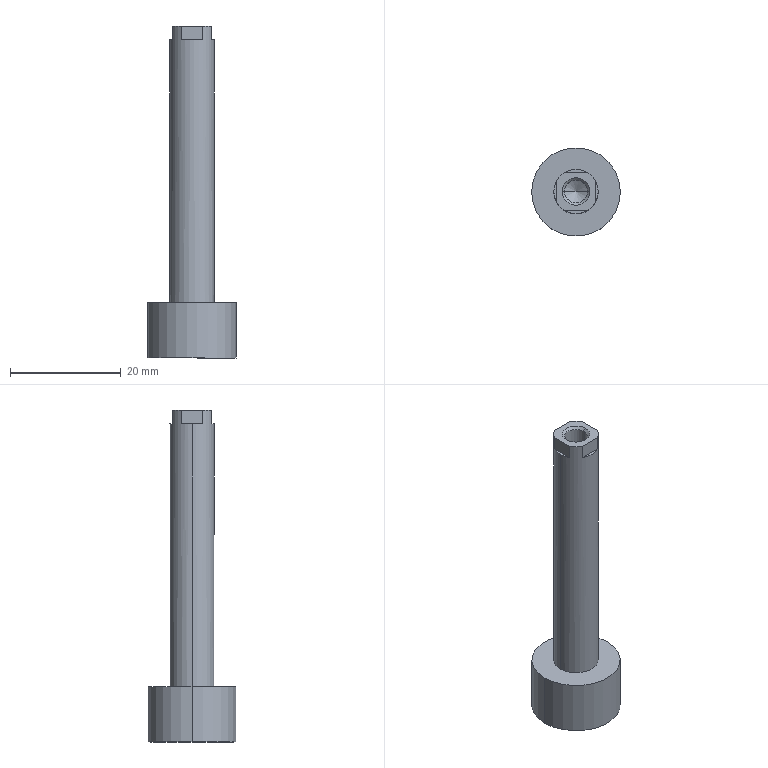Part | STEP file | 1 solid | 21 faces | box 16 x 16 x 60 mm | volume 4417 mm3 | plane 11 | cylinder 6 | cone 4 | commonest cylinder face diameters 4.134 x2 8 x2 16 x2
STEP:
#1=CARTESIAN_POINT('',(-4.,0.,-27.5));
#2=VERTEX_POINT('',#1);
#3=CARTESIAN_POINT('',(-4.,0.,20.));
#4=VERTEX_POINT('',#3);
#5=CARTESIAN_POINT('',(-4.,0.,-27.5));
#6=DIRECTION('',(0.,0.,1.));
#7=VECTOR('',#6,1000.);
#8=LINE('',#5,#7);
#9=EDGE_CURVE('',#2,#4,#8,.T.);
#10=ORIENTED_EDGE('',*,*,#9,.F.);
#11=CARTESIAN_POINT('',(4.,0.,-27.5));
#12=VERTEX_POINT('',#11);
#13=CARTESIAN_POINT('',(0.,0.,-27.5));
#14=DIRECTION('',(0.,0.,1.));
#15=DIRECTION('',(1.,0.,0.));
#16=AXIS2_PLACEMENT_3D('',#13,#14,#15);
#17=CIRCLE('',#16,4.);
#18=EDGE_CURVE('',#2,#12,#17,.T.);
#19=ORIENTED_EDGE('',*,*,#18,.T.);
#20=CARTESIAN_POINT('',(4.,0.,20.));
#21=VERTEX_POINT('',#20);
#22=CARTESIAN_POINT('',(4.,0.,-27.5));
#23=DIRECTION('',(0.,0.,1.));
#24=VECTOR('',#23,1000.);
#25=LINE('',#22,#24);
#26=EDGE_CURVE('',#12,#21,#25,.T.);
#27=ORIENTED_EDGE('',*,*,#26,.T.);
#28=CARTESIAN_POINT('',(3.5,-1.936,20.));
#29=VERTEX_POINT('',#28);
#30=CARTESIAN_POINT('',(0.,0.,20.));
#31=DIRECTION('',(0.,0.,1.));
#32=DIRECTION('',(1.,0.,0.));
#33=AXIS2_PLACEMENT_3D('',#30,#31,#32);
#34=CIRCLE('',#33,4.);
#35=EDGE_CURVE('',#29,#21,#34,.T.);
#36=ORIENTED_EDGE('',*,*,#35,.F.);
#37=CARTESIAN_POINT('',(3.5,-1.936,22.5));
#38=VERTEX_POINT('',#37);
#39=CARTESIAN_POINT('',(3.5,-1.936,22.5));
#40=DIRECTION('',(0.,0.,-1.));
#41=VECTOR('',#40,1000.);
#42=LINE('',#39,#41);
#43=EDGE_CURVE('',#38,#29,#42,.T.);
#44=ORIENTED_EDGE('',*,*,#43,.F.);
#45=CARTESIAN_POINT('',(1.936,-3.5,22.5));
#46=VERTEX_POINT('',#45);
#47=CARTESIAN_POINT('',(0.,0.,22.5));
#48=DIRECTION('',(0.,0.,1.));
#49=DIRECTION('',(1.,0.,0.));
#50=AXIS2_PLACEMENT_3D('',#47,#48,#49);
#51=CIRCLE('',#50,4.);
#52=EDGE_CURVE('',#46,#38,#51,.T.);
#53=ORIENTED_EDGE('',*,*,#52,.F.);
#54=CARTESIAN_POINT('',(1.936,-3.5,20.));
#55=VERTEX_POINT('',#54);
#56=CARTESIAN_POINT('',(1.936,-3.5,22.5));
#57=DIRECTION('',(0.,0.,1.));
#58=VECTOR('',#57,1000.);
#59=LINE('',#56,#58);
#60=EDGE_CURVE('',#55,#46,#59,.T.);
#61=ORIENTED_EDGE('',*,*,#60,.F.);
#62=CARTESIAN_POINT('',(-1.936,-3.5,20.));
#63=VERTEX_POINT('',#62);
#64=CARTESIAN_POINT('',(0.,0.,20.));
#65=DIRECTION('',(0.,0.,1.));
#66=DIRECTION('',(1.,0.,0.));
#67=AXIS2_PLACEMENT_3D('',#64,#65,#66);
#68=CIRCLE('',#67,4.);
#69=EDGE_CURVE('',#63,#55,#68,.T.);
#70=ORIENTED_EDGE('',*,*,#69,.F.);
#71=CARTESIAN_POINT('',(-1.936,-3.5,22.5));
#72=VERTEX_POINT('',#71);
#73=CARTESIAN_POINT('',(-1.936,-3.5,22.5));
#74=DIRECTION('',(0.,0.,-1.));
#75=VECTOR('',#74,1000.);
#76=LINE('',#73,#75);
#77=EDGE_CURVE('',#72,#63,#76,.T.);
#78=ORIENTED_EDGE('',*,*,#77,.F.);
#79=CARTESIAN_POINT('',(-3.5,-1.936,22.5));
#80=VERTEX_POINT('',#79);
#81=CARTESIAN_POINT('',(0.,0.,22.5));
#82=DIRECTION('',(0.,0.,1.));
#83=DIRECTION('',(1.,0.,0.));
#84=AXIS2_PLACEMENT_3D('',#81,#82,#83);
#85=CIRCLE('',#84,4.);
#86=EDGE_CURVE('',#80,#72,#85,.T.);
#87=ORIENTED_EDGE('',*,*,#86,.F.);
#88=CARTESIAN_POINT('',(-3.5,-1.936,20.));
#89=VERTEX_POINT('',#88);
#90=CARTESIAN_POINT('',(-3.5,-1.936,22.5));
#91=DIRECTION('',(0.,0.,1.));
#92=VECTOR('',#91,1000.);
#93=LINE('',#90,#92);
#94=EDGE_CURVE('',#89,#80,#93,.T.);
#95=ORIENTED_EDGE('',*,*,#94,.F.);
#96=CARTESIAN_POINT('',(0.,0.,20.));
#97=DIRECTION('',(0.,0.,1.));
#98=DIRECTION('',(1.,0.,0.));
#99=AXIS2_PLACEMENT_3D('',#96,#97,#98);
#100=CIRCLE('',#99,4.);
#101=EDGE_CURVE('',#4,#89,#100,.T.);
#102=ORIENTED_EDGE('',*,*,#101,.F.);
#103=EDGE_LOOP('',(#10,#19,#27,#36,#44,#53,#61,#70,#78,#87,#95,#102));
#104=FACE_OUTER_BOUND('',#103,.T.);
#105=CARTESIAN_POINT('',(0.,0.,22.5));
#106=DIRECTION('',(0.,0.,1.));
#107=DIRECTION('',(0.,1.,0.));
#108=AXIS2_PLACEMENT_3D('',#105,#106,#107);
#109=CYLINDRICAL_SURFACE('',#108,4.);
#110=ADVANCED_FACE('',(#104),#109,.T.);
#111=CARTESIAN_POINT('',(-3.5,1.936,20.));
#112=VERTEX_POINT('',#111);
#113=CARTESIAN_POINT('',(0.,0.,20.));
#114=DIRECTION('',(0.,0.,1.));
#115=DIRECTION('',(1.,0.,0.));
#116=AXIS2_PLACEMENT_3D('',#113,#114,#115);
#117=CIRCLE('',#116,4.);
#118=EDGE_CURVE('',#112,#4,#117,.T.);
#119=ORIENTED_EDGE('',*,*,#118,.T.);
#120=ORIENTED_EDGE('',*,*,#101,.T.);
#121=CARTESIAN_POINT('',(-3.5,3.5,20.));
#122=DIRECTION('',(0.,-1.,0.));
#123=VECTOR('',#122,1000.);
#124=LINE('',#121,#123);
#125=EDGE_CURVE('',#112,#89,#124,.T.);
#126=ORIENTED_EDGE('',*,*,#125,.F.);
#127=EDGE_LOOP('',(#119,#120,#126));
#128=FACE_OUTER_BOUND('',#127,.T.);
#129=CARTESIAN_POINT('',(0.,0.,20.));
#130=DIRECTION('',(0.,0.,1.));
#131=DIRECTION('',(1.,0.,0.));
#132=AXIS2_PLACEMENT_3D('',#129,#130,#131);
#133=PLANE('',#132);
#134=ADVANCED_FACE('',(#128),#133,.T.);
#135=ORIENTED_EDGE('',*,*,#94,.T.);
#136=CARTESIAN_POINT('',(-3.5,1.936,22.5));
#137=VERTEX_POINT('',#136);
#138=CARTESIAN_POINT('',(-3.5,3.5,22.5));
#139=DIRECTION('',(0.,-1.,0.));
#140=VECTOR('',#139,1000.);
#141=LINE('',#138,#140);
#142=EDGE_CURVE('',#137,#80,#141,.T.);
#143=ORIENTED_EDGE('',*,*,#142,.F.);
#144=CARTESIAN_POINT('',(-3.5,1.936,22.5));
#145=DIRECTION('',(0.,0.,-1.));
#146=VECTOR('',#145,1000.);
#147=LINE('',#144,#146);
#148=EDGE_CURVE('',#137,#112,#147,.T.);
#149=ORIENTED_EDGE('',*,*,#148,.T.);
#150=ORIENTED_EDGE('',*,*,#125,.T.);
#151=EDGE_LOOP('',(#135,#143,#149,#150));
#152=FACE_OUTER_BOUND('',#151,.T.);
#153=CARTESIAN_POINT('',(-3.5,3.5,20.));
#154=DIRECTION('',(-1.,0.,0.));
#155=DIRECTION('',(0.,0.,1.));
#156=AXIS2_PLACEMENT_3D('',#153,#154,#155);
#157=PLANE('',#156);
#158=ADVANCED_FACE('',(#152),#157,.T.);
#159=ORIENTED_EDGE('',*,*,#9,.T.);
#160=ORIENTED_EDGE('',*,*,#118,.F.);
#161=ORIENTED_EDGE('',*,*,#148,.F.);
#162=CARTESIAN_POINT('',(-1.936,3.5,22.5));
#163=VERTEX_POINT('',#162);
#164=CARTESIAN_POINT('',(0.,0.,22.5));
#165=DIRECTION('',(0.,0.,1.));
#166=DIRECTION('',(1.,0.,0.));
#167=AXIS2_PLACEMENT_3D('',#164,#165,#166);
#168=CIRCLE('',#167,4.);
#169=EDGE_CURVE('',#163,#137,#168,.T.);
#170=ORIENTED_EDGE('',*,*,#169,.F.);
#171=CARTESIAN_POINT('',(-1.936,3.5,20.));
#172=VERTEX_POINT('',#171);
#173=CARTESIAN_POINT('',(-1.936,3.5,22.5));
#174=DIRECTION('',(0.,0.,1.));
#175=VECTOR('',#174,1000.);
#176=LINE('',#173,#175);
#177=EDGE_CURVE('',#172,#163,#176,.T.);
#178=ORIENTED_EDGE('',*,*,#177,.F.);
#179=CARTESIAN_POINT('',(1.936,3.5,20.));
#180=VERTEX_POINT('',#179);
#181=CARTESIAN_POINT('',(0.,0.,20.));
#182=DIRECTION('',(0.,0.,1.));
#183=DIRECTION('',(1.,0.,0.));
#184=AXIS2_PLACEMENT_3D('',#181,#182,#183);
#185=CIRCLE('',#184,4.);
#186=EDGE_CURVE('',#180,#172,#185,.T.);
#187=ORIENTED_EDGE('',*,*,#186,.F.);
#188=CARTESIAN_POINT('',(1.936,3.5,22.5));
#189=VERTEX_POINT('',#188);
#190=CARTESIAN_POINT('',(1.936,3.5,22.5));
#191=DIRECTION('',(0.,0.,-1.));
#192=VECTOR('',#191,1000.);
#193=LINE('',#190,#192);
#194=EDGE_CURVE('',#189,#180,#193,.T.);
#195=ORIENTED_EDGE('',*,*,#194,.F.);
#196=CARTESIAN_POINT('',(3.5,1.936,22.5));
#197=VERTEX_POINT('',#196);
#198=CARTESIAN_POINT('',(0.,0.,22.5));
#199=DIRECTION('',(0.,0.,1.));
#200=DIRECTION('',(1.,0.,0.));
#201=AXIS2_PLACEMENT_3D('',#198,#199,#200);
#202=CIRCLE('',#201,4.);
#203=EDGE_CURVE('',#197,#189,#202,.T.);
#204=ORIENTED_EDGE('',*,*,#203,.F.);
#205=CARTESIAN_POINT('',(3.5,1.936,20.));
#206=VERTEX_POINT('',#205);
#207=CARTESIAN_POINT('',(3.5,1.936,22.5));
#208=DIRECTION('',(0.,0.,1.));
#209=VECTOR('',#208,1000.);
#210=LINE('',#207,#209);
#211=EDGE_CURVE('',#206,#197,#210,.T.);
#212=ORIENTED_EDGE('',*,*,#211,.F.);
#213=CARTESIAN_POINT('',(0.,0.,20.));
#214=DIRECTION('',(0.,0.,1.));
#215=DIRECTION('',(1.,0.,0.));
#216=AXIS2_PLACEMENT_3D('',#213,#214,#215);
#217=CIRCLE('',#216,4.);
#218=EDGE_CURVE('',#21,#206,#217,.T.);
#219=ORIENTED_EDGE('',*,*,#218,.F.);
#220=ORIENTED_EDGE('',*,*,#26,.F.);
#221=CARTESIAN_POINT('',(0.,0.,-27.5));
#222=DIRECTION('',(0.,0.,1.));
#223=DIRECTION('',(1.,0.,0.));
#224=AXIS2_PLACEMENT_3D('',#221,#222,#223);
#225=CIRCLE('',#224,4.);
#226=EDGE_CURVE('',#12,#2,#225,.T.);
#227=ORIENTED_EDGE('',*,*,#226,.T.);
#228=EDGE_LOOP('',(#159,#160,#161,#170,#178,#187,#195,#204,#212,#219,#220,#227));
#229=FACE_OUTER_BOUND('',#228,.T.);
#230=CARTESIAN_POINT('',(0.,0.,22.5));
#231=DIRECTION('',(0.,0.,1.));
#232=DIRECTION('',(0.,-1.,0.));
#233=AXIS2_PLACEMENT_3D('',#230,#231,#232);
#234=CYLINDRICAL_SURFACE('',#233,4.);
#235=ADVANCED_FACE('',(#229),#234,.T.);
#236=ORIENTED_EDGE('',*,*,#18,.F.);
#237=ORIENTED_EDGE('',*,*,#226,.F.);
#238=EDGE_LOOP('',(#236,#237));
#239=FACE_BOUND('',#238,.T.);
#240=CARTESIAN_POINT('',(8.,0.,-27.5));
#241=VERTEX_POINT('',#240);
#242=CARTESIAN_POINT('',(-8.,0.,-27.5));
#243=VERTEX_POINT('',#242);
#244=CARTESIAN_POINT('',(0.,0.,-27.5));
#245=DIRECTION('',(0.,0.,1.));
#246=DIRECTION('',(1.,0.,0.));
#247=AXIS2_PLACEMENT_3D('',#244,#245,#246);
#248=CIRCLE('',#247,8.);
#249=EDGE_CURVE('',#241,#243,#248,.T.);
#250=ORIENTED_EDGE('',*,*,#249,.T.);
#251=CARTESIAN_POINT('',(0.,0.,-27.5));
#252=DIRECTION('',(0.,0.,1.));
#253=DIRECTION('',(1.,0.,0.));
#254=AXIS2_PLACEMENT_3D('',#251,#252,#253);
#255=CIRCLE('',#254,8.);
#256=EDGE_CURVE('',#243,#241,#255,.T.);
#257=ORIENTED_EDGE('',*,*,#256,.T.);
#258=EDGE_LOOP('',(#250,#257));
#259=FACE_OUTER_BOUND('',#258,.T.);
#260=CARTESIAN_POINT('',(8.,0.,-27.5));
#261=DIRECTION('',(0.,0.,-1.));
#262=DIRECTION('',(-1.,0.,0.));
#263=AXIS2_PLACEMENT_3D('',#260,#261,#262);
#264=PLANE('',#263);
#265=ADVANCED_FACE('',(#239,#259),#264,.F.);
#266=CARTESIAN_POINT('',(-8.,0.,-37.5));
#267=VERTEX_POINT('',#266);
#268=CARTESIAN_POINT('',(-8.,0.,-37.5));
#269=DIRECTION('',(0.,0.,1.));
#270=VECTOR('',#269,1000.);
#271=LINE('',#268,#270);
#272=EDGE_CURVE('',#267,#243,#271,.T.);
#273=ORIENTED_EDGE('',*,*,#272,.F.);
#274=CARTESIAN_POINT('',(8.,0.,-37.5));
#275=VERTEX_POINT('',#274);
#276=CARTESIAN_POINT('',(0.,0.,-37.5));
#277=DIRECTION('',(0.,0.,1.));
#278=DIRECTION('',(1.,0.,0.));
#279=AXIS2_PLACEMENT_3D('',#276,#277,#278);
#280=CIRCLE('',#279,8.);
#281=EDGE_CURVE('',#267,#275,#280,.T.);
#282=ORIENTED_EDGE('',*,*,#281,.T.);
#283=CARTESIAN_POINT('',(8.,0.,-37.5));
#284=DIRECTION('',(0.,0.,1.));
#285=VECTOR('',#284,1000.);
#286=LINE('',#283,#285);
#287=EDGE_CURVE('',#275,#241,#286,.T.);
#288=ORIENTED_EDGE('',*,*,#287,.T.);
#289=ORIENTED_EDGE('',*,*,#256,.F.);
#290=EDGE_LOOP('',(#273,#282,#288,#289));
#291=FACE_OUTER_BOUND('',#290,.T.);
#292=CARTESIAN_POINT('',(0.,0.,22.5));
#293=DIRECTION('',(0.,0.,1.));
#294=DIRECTION('',(0.,1.,0.));
#295=AXIS2_PLACEMENT_3D('',#292,#293,#294);
#296=CYLINDRICAL_SURFACE('',#295,8.);
#297=ADVANCED_FACE('',(#291),#296,.T.);
#298=ORIENTED_EDGE('',*,*,#272,.T.);
#299=ORIENTED_EDGE('',*,*,#249,.F.);
#300=ORIENTED_EDGE('',*,*,#287,.F.);
#301=CARTESIAN_POINT('',(0.,0.,-37.5));
#302=DIRECTION('',(0.,0.,1.));
#303=DIRECTION('',(1.,0.,0.));
#304=AXIS2_PLACEMENT_3D('',#301,#302,#303);
#305=CIRCLE('',#304,8.);
#306=EDGE_CURVE('',#275,#267,#305,.T.);
#307=ORIENTED_EDGE('',*,*,#306,.T.);
#308=EDGE_LOOP('',(#298,#299,#300,#307));
#309=FACE_OUTER_BOUND('',#308,.T.);
#310=CARTESIAN_POINT('',(0.,0.,22.5));
#311=DIRECTION('',(0.,0.,1.));
#312=DIRECTION('',(0.,-1.,0.));
#313=AXIS2_PLACEMENT_3D('',#310,#311,#312);
#314=CYLINDRICAL_SURFACE('',#313,8.);
#315=ADVANCED_FACE('',(#309),#314,.T.);
#316=ORIENTED_EDGE('',*,*,#281,.F.);
#317=ORIENTED_EDGE('',*,*,#306,.F.);
#318=EDGE_LOOP('',(#316,#317));
#319=FACE_OUTER_BOUND('',#318,.T.);
#320=CARTESIAN_POINT('',(0.,0.,-37.5));
#321=DIRECTION('',(0.,0.,1.));
#322=DIRECTION('',(1.,0.,0.));
#323=AXIS2_PLACEMENT_3D('',#320,#321,#322);
#324=PLANE('',#323);
#325=ADVANCED_FACE('',(#319),#324,.F.);
#326=CARTESIAN_POINT('',(3.5,-3.5,20.));
#327=DIRECTION('',(0.,1.,0.));
#328=VECTOR('',#327,1000.);
#329=LINE('',#326,#328);
#330=EDGE_CURVE('',#29,#206,#329,.T.);
#331=ORIENTED_EDGE('',*,*,#330,.F.);
#332=ORIENTED_EDGE('',*,*,#35,.T.);
#333=ORIENTED_EDGE('',*,*,#218,.T.);
#334=EDGE_LOOP('',(#331,#332,#333));
#335=FACE_OUTER_BOUND('',#334,.T.);
#336=CARTESIAN_POINT('',(0.,0.,20.));
#337=DIRECTION('',(0.,0.,1.));
#338=DIRECTION('',(1.,0.,0.));
#339=AXIS2_PLACEMENT_3D('',#336,#337,#338);
#340=PLANE('',#339);
#341=ADVANCED_FACE('',(#335),#340,.T.);
#342=ORIENTED_EDGE('',*,*,#211,.T.);
#343=CARTESIAN_POINT('',(3.5,0.,22.5));
#344=DIRECTION('',(0.,-1.,0.));
#345=VECTOR('',#344,1000.);
#346=LINE('',#343,#345);
#347=EDGE_CURVE('',#197,#38,#346,.T.);
#348=ORIENTED_EDGE('',*,*,#347,.T.);
#349=ORIENTED_EDGE('',*,*,#43,.T.);
#350=ORIENTED_EDGE('',*,*,#330,.T.);
#351=EDGE_LOOP('',(#342,#348,#349,#350));
#352=FACE_OUTER_BOUND('',#351,.T.);
#353=CARTESIAN_POINT('',(3.5,-3.5,20.));
#354=DIRECTION('',(1.,0.,0.));
#355=DIRECTION('',(0.,0.,-1.));
#356=AXIS2_PLACEMENT_3D('',#353,#354,#355);
#357=PLANE('',#356);
#358=ADVANCED_FACE('',(#352),#357,.T.);
#359=CARTESIAN_POINT('',(-2.5,0.,22.5));
#360=VERTEX_POINT('',#359);
#361=CARTESIAN_POINT('',(2.5,0.,22.5));
#362=VERTEX_POINT('',#361);
#363=CARTESIAN_POINT('',(0.,0.,22.5));
#364=DIRECTION('',(0.,0.,1.));
#365=DIRECTION('',(1.,0.,0.));
#366=AXIS2_PLACEMENT_3D('',#363,#364,#365);
#367=CIRCLE('',#366,2.5);
#368=EDGE_CURVE('',#360,#362,#367,.T.);
#369=ORIENTED_EDGE('',*,*,#368,.F.);
#370=CARTESIAN_POINT('',(0.,0.,22.5));
#371=DIRECTION('',(0.,0.,1.));
#372=DIRECTION('',(1.,0.,0.));
#373=AXIS2_PLACEMENT_3D('',#370,#371,#372);
#374=CIRCLE('',#373,2.5);
#375=EDGE_CURVE('',#362,#360,#374,.T.);
#376=ORIENTED_EDGE('',*,*,#375,.F.);
#377=EDGE_LOOP('',(#369,#376));
#378=FACE_BOUND('',#377,.T.);
#379=ORIENTED_EDGE('',*,*,#142,.T.);
#380=ORIENTED_EDGE('',*,*,#86,.T.);
#381=CARTESIAN_POINT('',(-3.5,-3.5,22.5));
#382=DIRECTION('',(1.,0.,0.));
#383=VECTOR('',#382,1000.);
#384=LINE('',#381,#383);
#385=EDGE_CURVE('',#72,#46,#384,.T.);
#386=ORIENTED_EDGE('',*,*,#385,.T.);
#387=ORIENTED_EDGE('',*,*,#52,.T.);
#388=ORIENTED_EDGE('',*,*,#347,.F.);
#389=ORIENTED_EDGE('',*,*,#203,.T.);
#390=CARTESIAN_POINT('',(3.5,3.5,22.5));
#391=DIRECTION('',(-1.,0.,0.));
#392=VECTOR('',#391,1000.);
#393=LINE('',#390,#392);
#394=EDGE_CURVE('',#189,#163,#393,.T.);
#395=ORIENTED_EDGE('',*,*,#394,.T.);
#396=ORIENTED_EDGE('',*,*,#169,.T.);
#397=EDGE_LOOP('',(#379,#380,#386,#387,#388,#389,#395,#396));
#398=FACE_OUTER_BOUND('',#397,.T.);
#399=CARTESIAN_POINT('',(4.,0.,22.5));
#400=DIRECTION('',(0.,0.,-1.));
#401=DIRECTION('',(-1.,0.,0.));
#402=AXIS2_PLACEMENT_3D('',#399,#400,#401);
#403=PLANE('',#402);
#404=ADVANCED_FACE('',(#378,#398),#403,.F.);
#405=ORIENTED_EDGE('',*,*,#177,.T.);
#406=ORIENTED_EDGE('',*,*,#394,.F.);
#407=ORIENTED_EDGE('',*,*,#194,.T.);
#408=CARTESIAN_POINT('',(3.5,3.5,20.));
#409=DIRECTION('',(-1.,0.,0.));
#410=VECTOR('',#409,1000.);
#411=LINE('',#408,#410);
#412=EDGE_CURVE('',#180,#172,#411,.T.);
#413=ORIENTED_EDGE('',*,*,#412,.T.);
#414=EDGE_LOOP('',(#405,#406,#407,#413));
#415=FACE_OUTER_BOUND('',#414,.T.);
#416=CARTESIAN_POINT('',(3.5,3.5,20.));
#417=DIRECTION('',(0.,1.,0.));
#418=DIRECTION('',(0.,0.,1.));
#419=AXIS2_PLACEMENT_3D('',#416,#417,#418);
#420=PLANE('',#419);
#421=ADVANCED_FACE('',(#415),#420,.T.);
#422=ORIENTED_EDGE('',*,*,#186,.T.);
#423=ORIENTED_EDGE('',*,*,#412,.F.);
#424=EDGE_LOOP('',(#422,#423));
#425=FACE_OUTER_BOUND('',#424,.T.);
#426=CARTESIAN_POINT('',(0.,0.,20.));
#427=DIRECTION('',(0.,0.,1.));
#428=DIRECTION('',(1.,0.,0.));
#429=AXIS2_PLACEMENT_3D('',#426,#427,#428);
#430=PLANE('',#429);
#431=ADVANCED_FACE('',(#425),#430,.T.);
#432=ORIENTED_EDGE('',*,*,#60,.T.);
#433=ORIENTED_EDGE('',*,*,#385,.F.);
#434=ORIENTED_EDGE('',*,*,#77,.T.);
#435=CARTESIAN_POINT('',(-3.5,-3.5,20.));
#436=DIRECTION('',(1.,0.,0.));
#437=VECTOR('',#436,1000.);
#438=LINE('',#435,#437);
#439=EDGE_CURVE('',#63,#55,#438,.T.);
#440=ORIENTED_EDGE('',*,*,#439,.T.);
#441=EDGE_LOOP('',(#432,#433,#434,#440));
#442=FACE_OUTER_BOUND('',#441,.T.);
#443=CARTESIAN_POINT('',(-3.5,-3.5,20.));
#444=DIRECTION('',(0.,-1.,0.));
#445=DIRECTION('',(0.,0.,-1.));
#446=AXIS2_PLACEMENT_3D('',#443,#444,#445);
#447=PLANE('',#446);
#448=ADVANCED_FACE('',(#442),#447,.T.);
#449=ORIENTED_EDGE('',*,*,#69,.T.);
#450=ORIENTED_EDGE('',*,*,#439,.F.);
#451=EDGE_LOOP('',(#449,#450));
#452=FACE_OUTER_BOUND('',#451,.T.);
#453=CARTESIAN_POINT('',(0.,0.,20.));
#454=DIRECTION('',(0.,0.,1.));
#455=DIRECTION('',(1.,0.,0.));
#456=AXIS2_PLACEMENT_3D('',#453,#454,#455);
#457=PLANE('',#456);
#458=ADVANCED_FACE('',(#452),#457,.T.);
#459=CARTESIAN_POINT('',(-2.067,0.,22.067));
#460=VERTEX_POINT('',#459);
#461=CARTESIAN_POINT('',(-2.067,0.,22.067));
#462=DIRECTION('',(-0.7071,0.,0.7071));
#463=VECTOR('',#462,1000.);
#464=LINE('',#461,#463);
#465=EDGE_CURVE('',#460,#360,#464,.T.);
#466=ORIENTED_EDGE('',*,*,#465,.F.);
#467=CARTESIAN_POINT('',(2.067,0.,22.067));
#468=VERTEX_POINT('',#467);
#469=CARTESIAN_POINT('',(0.,0.,22.067));
#470=DIRECTION('',(0.,0.,1.));
#471=DIRECTION('',(1.,0.,0.));
#472=AXIS2_PLACEMENT_3D('',#469,#470,#471);
#473=CIRCLE('',#472,2.067);
#474=EDGE_CURVE('',#468,#460,#473,.T.);
#475=ORIENTED_EDGE('',*,*,#474,.F.);
#476=CARTESIAN_POINT('',(2.067,0.,22.067));
#477=DIRECTION('',(0.7071,0.,0.7071));
#478=VECTOR('',#477,1000.);
#479=LINE('',#476,#478);
#480=EDGE_CURVE('',#468,#362,#479,.T.);
#481=ORIENTED_EDGE('',*,*,#480,.T.);
#482=ORIENTED_EDGE('',*,*,#375,.T.);
#483=EDGE_LOOP('',(#466,#475,#481,#482));
#484=FACE_OUTER_BOUND('',#483,.T.);
#485=CARTESIAN_POINT('',(0.,0.,22.5));
#486=DIRECTION('',(0.,0.,1.));
#487=DIRECTION('',(0.,-1.,0.));
#488=AXIS2_PLACEMENT_3D('',#485,#486,#487);
#489=CONICAL_SURFACE('',#488,2.5,0.7854);
#490=ADVANCED_FACE('',(#484),#489,.F.);
#491=ORIENTED_EDGE('',*,*,#465,.T.);
#492=ORIENTED_EDGE('',*,*,#368,.T.);
#493=ORIENTED_EDGE('',*,*,#480,.F.);
#494=CARTESIAN_POINT('',(0.,0.,22.067));
#495=DIRECTION('',(0.,0.,1.));
#496=DIRECTION('',(1.,0.,0.));
#497=AXIS2_PLACEMENT_3D('',#494,#495,#496);
#498=CIRCLE('',#497,2.067);
#499=EDGE_CURVE('',#460,#468,#498,.T.);
#500=ORIENTED_EDGE('',*,*,#499,.F.);
#501=EDGE_LOOP('',(#491,#492,#493,#500));
#502=FACE_OUTER_BOUND('',#501,.T.);
#503=CARTESIAN_POINT('',(0.,0.,22.5));
#504=DIRECTION('',(0.,0.,1.));
#505=DIRECTION('',(0.,1.,0.));
#506=AXIS2_PLACEMENT_3D('',#503,#504,#505);
#507=CONICAL_SURFACE('',#506,2.5,0.7854);
#508=ADVANCED_FACE('',(#502),#507,.F.);
#509=CARTESIAN_POINT('',(-2.067,0.,16.));
#510=VERTEX_POINT('',#509);
#511=CARTESIAN_POINT('',(-2.067,0.,16.));
#512=DIRECTION('',(0.,0.,1.));
#513=VECTOR('',#512,1000.);
#514=LINE('',#511,#513);
#515=EDGE_CURVE('',#510,#460,#514,.T.);
#516=ORIENTED_EDGE('',*,*,#515,.T.);
#517=ORIENTED_EDGE('',*,*,#499,.T.);
#518=CARTESIAN_POINT('',(2.067,0.,16.));
#519=VERTEX_POINT('',#518);
#520=CARTESIAN_POINT('',(2.067,0.,16.));
#521=DIRECTION('',(0.,0.,1.));
#522=VECTOR('',#521,1000.);
#523=LINE('',#520,#522);
#524=EDGE_CURVE('',#519,#468,#523,.T.);
#525=ORIENTED_EDGE('',*,*,#524,.F.);
#526=CARTESIAN_POINT('',(0.,0.,16.));
#527=DIRECTION('',(0.,0.,1.));
#528=DIRECTION('',(1.,0.,0.));
#529=AXIS2_PLACEMENT_3D('',#526,#527,#528);
#530=CIRCLE('',#529,2.067);
#531=EDGE_CURVE('',#510,#519,#530,.T.);
#532=ORIENTED_EDGE('',*,*,#531,.F.);
#533=EDGE_LOOP('',(#516,#517,#525,#532));
#534=FACE_OUTER_BOUND('',#533,.T.);
#535=CARTESIAN_POINT('',(0.,0.,22.5));
#536=DIRECTION('',(0.,0.,1.));
#537=DIRECTION('',(0.,1.,0.));
#538=AXIS2_PLACEMENT_3D('',#535,#536,#537);
#539=CYLINDRICAL_SURFACE('',#538,2.067);
#540=ADVANCED_FACE('',(#534),#539,.F.);
#541=CARTESIAN_POINT('',(0.,0.,14.807));
#542=VERTEX_POINT('',#541);
#543=CARTESIAN_POINT('',(0.,0.,14.807));
#544=DIRECTION('',(-0.866,0.,0.5));
#545=VECTOR('',#544,1000.);
#546=LINE('',#543,#545);
#547=EDGE_CURVE('',#542,#510,#546,.T.);
#548=ORIENTED_EDGE('',*,*,#547,.T.);
#549=ORIENTED_EDGE('',*,*,#531,.T.);
#550=CARTESIAN_POINT('',(0.,0.,14.807));
#551=DIRECTION('',(0.866,0.,0.5));
#552=VECTOR('',#551,1000.);
#553=LINE('',#550,#552);
#554=EDGE_CURVE('',#542,#519,#553,.T.);
#555=ORIENTED_EDGE('',*,*,#554,.F.);
#556=EDGE_LOOP('',(#548,#549,#555));
#557=FACE_OUTER_BOUND('',#556,.T.);
#558=CARTESIAN_POINT('',(0.,0.,16.));
#559=DIRECTION('',(0.,0.,1.));
#560=DIRECTION('',(0.,1.,0.));
#561=AXIS2_PLACEMENT_3D('',#558,#559,#560);
#562=CONICAL_SURFACE('',#561,2.067,1.047);
#563=ADVANCED_FACE('',(#557),#562,.F.);
#564=ORIENTED_EDGE('',*,*,#554,.T.);
#565=CARTESIAN_POINT('',(0.,0.,16.));
#566=DIRECTION('',(0.,0.,1.));
#567=DIRECTION('',(1.,0.,0.));
#568=AXIS2_PLACEMENT_3D('',#565,#566,#567);
#569=CIRCLE('',#568,2.067);
#570=EDGE_CURVE('',#519,#510,#569,.T.);
#571=ORIENTED_EDGE('',*,*,#570,.T.);
#572=ORIENTED_EDGE('',*,*,#547,.F.);
#573=EDGE_LOOP('',(#564,#571,#572));
#574=FACE_OUTER_BOUND('',#573,.T.);
#575=CARTESIAN_POINT('',(0.,0.,16.));
#576=DIRECTION('',(0.,0.,1.));
#577=DIRECTION('',(0.,-1.,0.));
#578=AXIS2_PLACEMENT_3D('',#575,#576,#577);
#579=CONICAL_SURFACE('',#578,2.067,1.047);
#580=ADVANCED_FACE('',(#574),#579,.F.);
#581=ORIENTED_EDGE('',*,*,#515,.F.);
#582=ORIENTED_EDGE('',*,*,#570,.F.);
#583=ORIENTED_EDGE('',*,*,#524,.T.);
#584=ORIENTED_EDGE('',*,*,#474,.T.);
#585=EDGE_LOOP('',(#581,#582,#583,#584));
#586=FACE_OUTER_BOUND('',#585,.T.);
#587=CARTESIAN_POINT('',(0.,0.,22.5));
#588=DIRECTION('',(0.,0.,1.));
#589=DIRECTION('',(0.,-1.,0.));
#590=AXIS2_PLACEMENT_3D('',#587,#588,#589);
#591=CYLINDRICAL_SURFACE('',#590,2.067);
#592=ADVANCED_FACE('',(#586),#591,.F.);
#593=CLOSED_SHELL('',(#110,#134,#158,#235,#265,#297,#315,#325,#341,#358,#404,#421,#431,#448,#458,#490,#508,#540,#563,#580,#592));
#594=MANIFOLD_SOLID_BREP('',#593);
#595=CARTESIAN_POINT('',(0.,0.,0.));
#596=DIRECTION('',(0.,0.,1.));
#597=DIRECTION('',(1.,0.,0.));
#598=AXIS2_PLACEMENT_3D('',#595,#596,#597);
#599=(LENGTH_UNIT()NAMED_UNIT(*)SI_UNIT(.MILLI.,.METRE.));
#600=UNCERTAINTY_MEASURE_WITH_UNIT(LENGTH_MEASURE(0.00001),#599,'','');
#601=(NAMED_UNIT(*)PLANE_ANGLE_UNIT()SI_UNIT($,.RADIAN.));
#602=(NAMED_UNIT(*)SI_UNIT($,.STERADIAN.)SOLID_ANGLE_UNIT());
#603=(GEOMETRIC_REPRESENTATION_CONTEXT(3)GLOBAL_UNCERTAINTY_ASSIGNED_CONTEXT((#600))GLOBAL_UNIT_ASSIGNED_CONTEXT((#599,#601,#602))REPRESENTATION_CONTEXT('',''));
#604=ADVANCED_BREP_SHAPE_REPRESENTATION('',(#594,#598),#603);